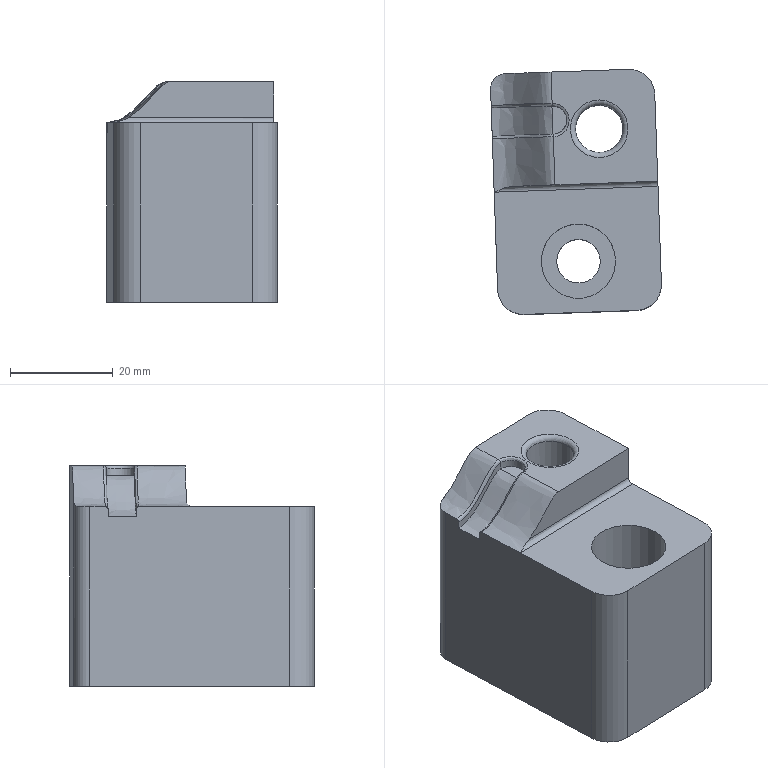Part | NX | features DIE-64 2 | 1 solid | 30 faces | box 33.293 x 47.743 x 43 mm | volume 49196 mm3 | plane 11 | spline 9 | cylinder 9 | torus 1 | commonest cylinder face diameters 10 x3 2 x1 6 x1 8.5 x1 9.24 x1 14 x1